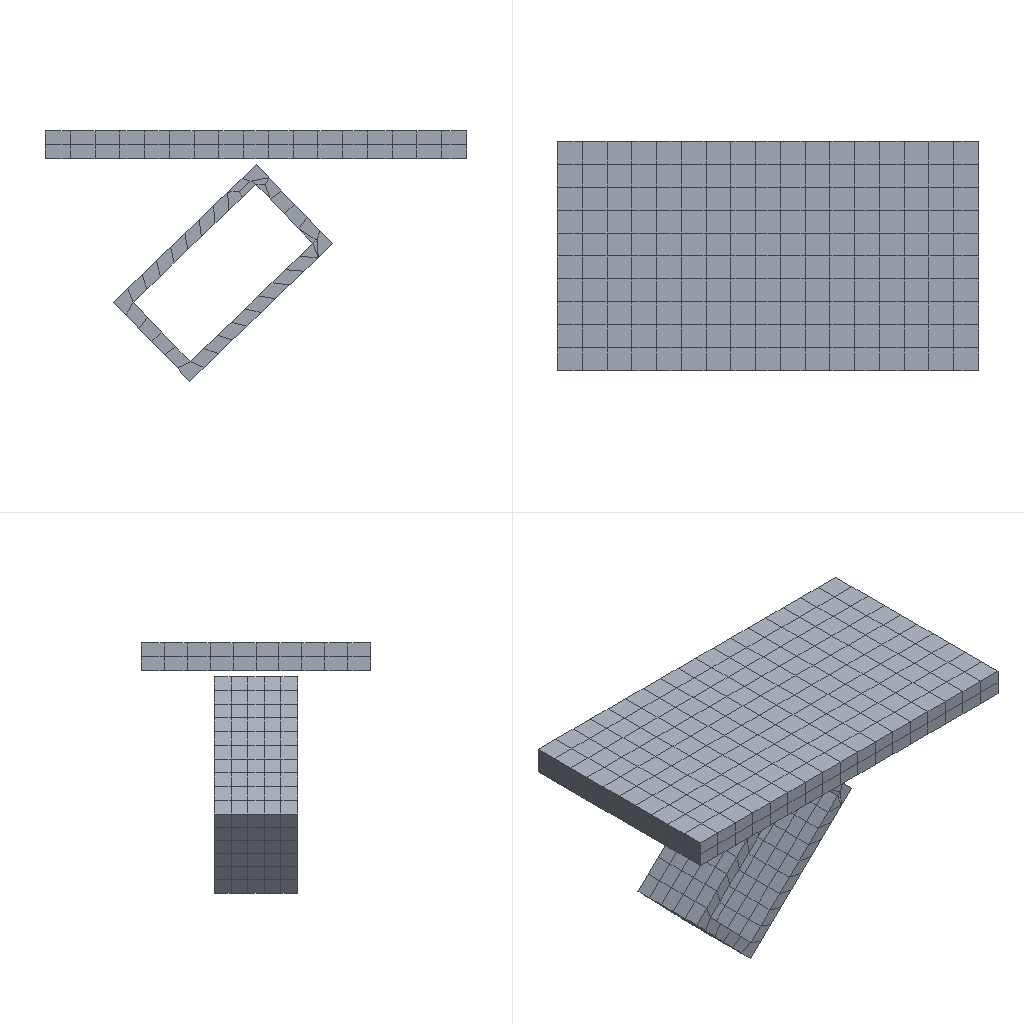Simulation study | ansys workbench
Set-up summary:
category,name,step,type,value,unit,region
solver,ansys_workbench
units,mm-N-s-tonne (MPa),,stated,"/units,MPA"
analysis,LS1,,transient
load_step,LS1,LS1,transient,time=5
mesh,nodes,,,3355
mesh,elements,,,515
element_type,SOLID186,,,515
material,Structural Steel,,E,200000,tonne s^-2 mm^-1
material,Structural Steel,,nu,0.3
material,Structural Steel,,density,7.85e-09,tonne mm^-3
material,Structural Steel,,conductivity,60.5,tonne mm s^-3 C^-1
material,Structural Steel,,specific_heat,4.34e+08,mm^2 s^-2 C^-1
material,Structural Steel,,cte,1.2e-05,C^-1
material,Structural Steel,,permeability,10000
material,Structural Steel,,resistivity,0.00017,ohm mm
bc,Fixed Supports,model,fixed,[dofs=ALL],,_FIXEDSU
bc,Send Velocity Tables and Functions * Components,LS1,prescribed velz,10 [dofs=VELZ],,_CM35VELZ_ZP
named_set,_FIXEDSU,,node,565
named_set,_CM35VELZ_ZP,,node,164
Ansys APDL input file, long lists of numbers shortened:
/batch
/config,noeldb,1     ! force off writing results to database
*get,_wallstrt,active,,time,wall
! ANSYS input file written by Workbench version 2022 R1
! File used for geometry attach:
/title,wbnew--__ (A5)
! ****** Begin Custom Load Command Snippet ******
/COM, ACT Extensions:
/COM,     LSDYNA, 2021.1
/COM,
! ****** End   Custom Load Command Snippet ******
*DIM,_wb_ProjectScratch_dir,string,248
_wb_ProjectScratch_dir(1) = ''
*DIM,_wb_SolverFiles_dir,string,248
_wb_SolverFiles_dir(1) = ''
*DIM,_wb_userfiles_dir,string,248
_wb_userfiles_dir(1) = ''
/com,--- Data in consistent NMM units. See Solving Units in the help system for more information.
/units,MPA
/nopr
/wb,file,start              !  signify a WB generated input file
/prep7
! Turn off shape checking because checks already performed inside WB mesher.
! See help system for more information.
SHPP,OFF,,NOWARN
/nolist
etcon,set             ! allow ANSYS to choose best KEYOP's for 180x elements, resets any applicable keyopt to MAPDL defaults
/com,*********** Nodes for the whole assembly ***********
nblock,3,,3690
(1i9,3e20.9e3)
        1    -6.708473777E+01     3.315979729E+01     5.000000000E+00
! (3354 more lines like these left out)
-1
/wb,elem,start            !  set before creation of elements
/com,*********** Elements for Body 1 "__1-FreeParts|__-__2" ***********
et,1,186
keyo,1,2,1          ! set full integration on SOLID186
eblock,19,solid,,175
(19i9)
        1        1        1        1        0        0        0        0       20        0      341     2096     2232     2104     2382     2110     2249     2108     2383
! (349 more lines like these left out)
-1
/com,*********** Elements for Body 2 "__1-FreeParts|__-__1" ***********
et,2,186
keyo,2,2,1          ! set full integration on SOLID186
eblock,19,solid,,340
(19i9)
        2        2        2        2        0        0        0        0       20        0        1        1      551      542      509      288      552      541      540
! (679 more lines like these left out)
-1
/wb,elem,end               !  done creating elements
/com,*********** Send User Defined Coordinate System(s) ***********
csys,0
toffst,273.15,  ! Temperature offset from absolute zero
/com,*********** Set Reference Temperature ***********
tref,22.
/wb,mat,start              !  starting to send materials
/com,*********** Send Materials ***********
Temperature = 'TEMP' ! Temperature
MP,DENS,1,7.85e-09,	! tonne mm^-3
MP,ALPX,1,1.2e-05,	! C^-1
MP,C,1,434000000,	! mm^2 s^-2 C^-1
MP,KXX,1,60.5,	! tonne mm s^-3 C^-1
MP,RSVX,1,0.00017,	! ohm mm
MP,EX,1,200000,	! tonne s^-2 mm^-1
MP,NUXY,1,0.3,
MP,MURX,1,10000,
Temperature = 'TEMP' ! Temperature
MP,DENS,2,7.85e-09,	! tonne mm^-3
MP,ALPX,2,1.2e-05,	! C^-1
MP,C,2,434000000,	! mm^2 s^-2 C^-1
MP,KXX,2,60.5,	! tonne mm s^-3 C^-1
MP,RSVX,2,0.00017,	! ohm mm
MP,EX,2,200000,	! tonne s^-2 mm^-1
MP,NUXY,2,0.3,
MP,MURX,2,10000,
/wb,mat,end                !  done sending materials
!************************* Model Summary ********************
!__1-FreeParts|__-__2,	结构钢,	matid,	1
!__1-FreeParts|__-__1,	结构钢,	matid,	2
!************************* End Model Summary ********************
! get the diagonal of the bounding box. Needed later for other things
*get,_xmin,node,,mnloc,x
*get,_ymin,node,,mnloc,y
*get,_zmin,node,,mnloc,z
*get,_xmax,node,,mxloc,x
*get,_ymax,node,,mxloc,y
*get,_zmax,node,,mxloc,z
_ASMDIAG=(_xmax-_xmin)*(_xmax-_xmin)+(_ymax-_ymin)*(_ymax-_ymin)+(_zmax-_zmin)*(_zmax-_zmin)
_ASMDIAG=SQRT(_ASMDIAG)
/wb,contact,start          !  starting to send contact
/wb,contact,end            !  done creating contacts
/golist
/wb,load,start             !  starting to send loads
/com,*********** Fixed Supports ***********
CMBLOCK,_FIXEDSU,NODE,      565
(8i10)
       289       290       291       292       293       294       295       296
! (70 more lines like these left out)
cmsel,s,_FIXEDSU
d,all,all
nsel,all
/gst,on,on
fini
*get,_numnode,node,0,count
*get,_numelem,elem,0,count
*get, _MAXELEMNUM, elem, 0, NUM, MAX
*get, _MAXNODENUM, node, 0, NUM, MAX
*get, _MAXELEMTYPE, etyp, 0, NUM, MAX
*get, _MAXREALCONST, real, 0, NUM, MAX
/go
/wb,load,end               !  done creating loads
/com,--- Number of total nodes = %_numnode%
/com,--- Number of contact elements = 0
/com,--- Number of spring elements = 0
/com,--- Number of bearing elements = 0
/com,--- Number of solid elements = 515
/com,--- Number of condensed parts = 0
/com,--- Number of total elements = %_numelem%
*get,_wallbsol,active,,time,wall
/com,****************************************************************************
/com,*************************    SOLUTION       ********************************
/com,****************************************************************************
/solu
antype,4                   ! transient analysis
nlgeom,on                  ! Turn on Large Deformation Effects
kbc,1                      ! stepped BC's
_thickRatio=  0     ! Ratio of thick parts in the model
eqsl,sparse,,,,,1
cntr,print,1               ! print out contact info and also make no initial contact an error
dmpoption,emat,no             ! Don't combine emat file for DANSYS
dmpoption,esav,no             ! Don't combine esav file for DANSYS
trnopt,full,,,,,hht        ! HHT time integration method
tintp, mosp			! Choose transient integration settings for moderate speed application
nldiag,cont,iter           ! print out contact info each equilibrium iteration
rescontrol,define,last,last,,dele	   ! Program Controlled
/com,****************************************************
/com,******************* SOLVE FOR LS 1 OF 1 ****************
/com,*** Send Velocity Tables and Functions * Components ***
CMBLOCK,_CM35VELZ_ZP,NODE,      164
(8i10)
      2132      2133      2134      2135      2136      2137      2138      2139
! (20 more lines like these left out)
cmsel,s,_CM35VELZ_ZP
d,all,velz,10.
nsel,all
/nopr
/gopr
autots,on                   ! User turned on automatic time stepping
deltim,1,1,1,OFF
time,5.
timint,on                  ! Turn on time integration effects
outres,erase
outres,all,none
outres,nsol,all,
outres,rsol,all
outres,eangl,all
outres,etmp,all
outres,veng,all
outres,strs,all,
outres,epel,all,
outres,eppl,all,
outres,cont,all,
outres,v,all,
outres,a,all,
! *********** WB SOLVE COMMAND ***********
! check interactive state
*get,ANSINTER_,active,,int
*if,ANSINTER_,ne,0,then
/eof
*endif
solve
/com *************** Write FE CONNECTORS *********
CEWRITE,file,ce,,INTE
/com,****************************************************
/com,*************** FINISHED SOLVE FOR LS 1 *************
*get,_wallasol,active,,time,wall
/nopr
*get,_numnode,node,0,count
*get,_numelem,elem,0,count
*get, _MAXELEMNUM, elem, 0, NUM, MAX
*get, _MAXNODENUM, node, 0, NUM, MAX,,,INTERNAL
*get, _MAXELEMTYPE, etyp, 0, NUM, MAX
*get, _MAXREALCONST, real, 0, NUM, MAX
/gopr
/post1
xmlo,ENCODING,ISO-8859-1
xmlo,parm
/xml,parm,xml
fini
/gopr
*get,_walldone,active,,time,wall
_preptime=(_wallbsol-_wallstrt)*3600
_solvtime=(_wallasol-_wallbsol)*3600
_posttime=(_walldone-_wallasol)*3600
_totaltim=(_walldone-_wallstrt)*3600
*get,_dlbratio,active,0,solu,dlbr
*get,_combtime,active,0,solu,comb
*get,_ssmode,active,0,solu,ssmm
*get,_ndofs,active,0,solu,ndof
*get,_sol_end_time,active,0,set,time
*if,_sol_end_time,eq,5.,then
/fclean				!clean distributed files
*endif
/com,--- Total number of nodes = %_numnode%
/com,--- Total number of elements = %_numelem%
/com,--- Element load balance ratio = %_dlbratio%
/com,--- Time to combine distributed files = %_combtime%
/com,--- Sparse memory mode = %_ssmode%
/com,--- Number of DOF = %_ndofs%
/wb,file,end               ! done with WB generated input
Results summary:
result,analyses[0].index,,,1
result,analyses[0].system,,,SYS
result,analyses[0].deck,,,deck.dat
result,analyses[0].solve_status,,,completed
result,analyses[0].analysis_type,,,static
result,analyses[0].physics,,,mechanical
result,analyses[0].unit_system,,,"NMM: mm, ton, N, s, mV, mA, degC"
result,analyses[0].n_sets,,,5
result,analyses[0].load_steps[0].set,set=5,,5
result,analyses[0].load_steps[0].time_or_freq,set=5,,5
result,analyses[0].load_steps[0].max_displacement_magnitude,set=5,,50
result,analyses[0].load_steps[0].max_von_mises_nodal,set=5,,0.0006668
result,analyses[0].load_steps[0].reaction_force_sum_xyz[1],set=5,,0
result,analyses[0].load_steps[0].reaction_force_sum_xyz[2],set=5,,0
result,analyses[0].load_steps[0].reaction_force_sum_xyz[3],set=5,,0.02086